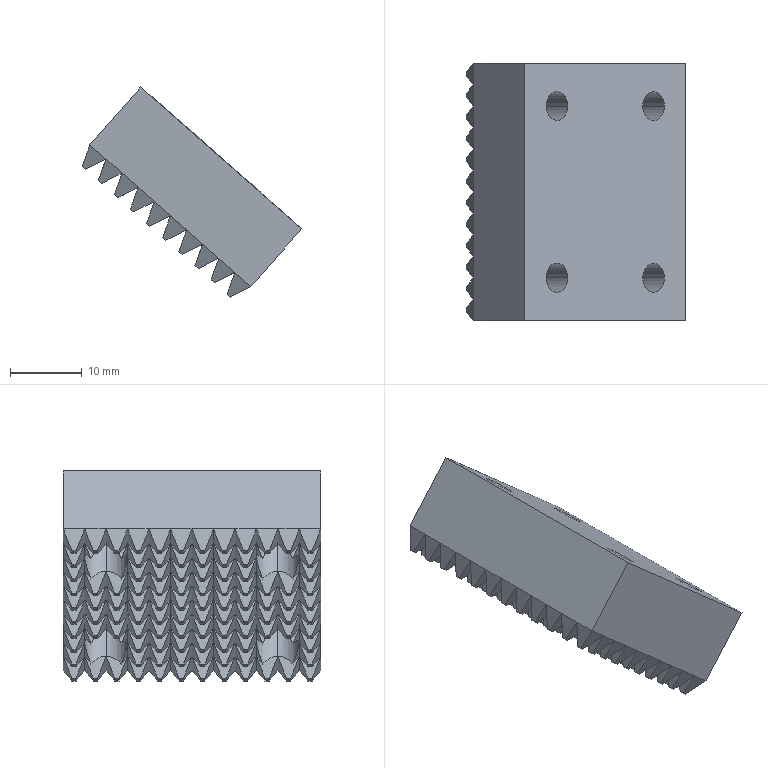Part | STEP file | 2026.6.15-Main Assembly图.sldasm-Part-189 | 1 solid | 577 faces | box 30.721 x 36 x 29.365 mm | volume 11937 mm3 | plane 561 | cylinder 16 | commonest cylinder face diameters 4.05 x8 6 x8